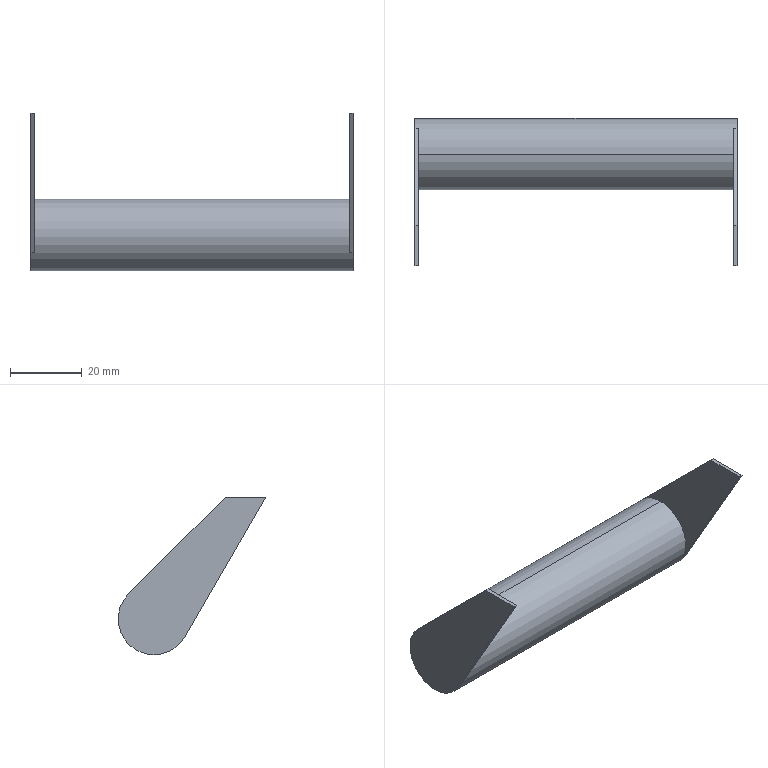Part | SolidWorks | features Extrusion 1, ICE 1, MirrorPattern 1 | 1 solid | 16 faces | box 90 x 41.177 x 44 mm | volume 6809 mm3 | plane 12 | cylinder 4 | commonest cylinder face diameters 18 x2 20 x2
STEP:
#1=CARTESIAN_POINT('',(45.,0.,-10.));
#2=VERTEX_POINT('',#1);
#3=CARTESIAN_POINT('',(45.,7.071,7.071));
#4=VERTEX_POINT('',#3);
#5=CARTESIAN_POINT('',(45.,0.,0.));
#6=DIRECTION('',(1.,0.,0.));
#7=DIRECTION('',(0.,0.,-1.));
#8=AXIS2_PLACEMENT_3D('',#5,#6,#7);
#9=CIRCLE('',#8,10.);
#10=EDGE_CURVE('',#2,#4,#9,.T.);
#11=ORIENTED_EDGE('',*,*,#10,.F.);
#12=CARTESIAN_POINT('',(-45.,0.,-10.));
#13=VERTEX_POINT('',#12);
#14=CARTESIAN_POINT('',(45.,0.,-10.));
#15=DIRECTION('',(-1.,0.,0.));
#16=VECTOR('',#15,1000.);
#17=LINE('',#14,#16);
#18=EDGE_CURVE('',#2,#13,#17,.T.);
#19=ORIENTED_EDGE('',*,*,#18,.T.);
#20=CARTESIAN_POINT('',(-45.,7.071,7.071));
#21=VERTEX_POINT('',#20);
#22=CARTESIAN_POINT('',(-45.,0.,0.));
#23=DIRECTION('',(1.,0.,0.));
#24=DIRECTION('',(0.,0.,-1.));
#25=AXIS2_PLACEMENT_3D('',#22,#23,#24);
#26=CIRCLE('',#25,10.);
#27=EDGE_CURVE('',#13,#21,#26,.T.);
#28=ORIENTED_EDGE('',*,*,#27,.T.);
#29=CARTESIAN_POINT('',(-44.,7.071,7.071));
#30=VERTEX_POINT('',#29);
#31=CARTESIAN_POINT('',(-44.,7.071,7.071));
#32=DIRECTION('',(-1.,0.,0.));
#33=VECTOR('',#32,1000.);
#34=LINE('',#31,#33);
#35=EDGE_CURVE('',#30,#21,#34,.T.);
#36=ORIENTED_EDGE('',*,*,#35,.F.);
#37=CARTESIAN_POINT('',(-44.,0.,10.));
#38=VERTEX_POINT('',#37);
#39=CARTESIAN_POINT('',(-44.,0.,0.));
#40=DIRECTION('',(-1.,0.,0.));
#41=DIRECTION('',(0.,0.,1.));
#42=AXIS2_PLACEMENT_3D('',#39,#40,#41);
#43=CIRCLE('',#42,10.);
#44=EDGE_CURVE('',#38,#30,#43,.T.);
#45=ORIENTED_EDGE('',*,*,#44,.F.);
#46=CARTESIAN_POINT('',(44.,0.,10.));
#47=VERTEX_POINT('',#46);
#48=CARTESIAN_POINT('',(45.,0.,10.));
#49=DIRECTION('',(-1.,0.,0.));
#50=VECTOR('',#49,1000.);
#51=LINE('',#48,#50);
#52=EDGE_CURVE('',#47,#38,#51,.T.);
#53=ORIENTED_EDGE('',*,*,#52,.F.);
#54=CARTESIAN_POINT('',(44.,7.071,7.071));
#55=VERTEX_POINT('',#54);
#56=CARTESIAN_POINT('',(44.,0.,0.));
#57=DIRECTION('',(1.,0.,0.));
#58=DIRECTION('',(0.,0.,-1.));
#59=AXIS2_PLACEMENT_3D('',#56,#57,#58);
#60=CIRCLE('',#59,10.);
#61=EDGE_CURVE('',#55,#47,#60,.T.);
#62=ORIENTED_EDGE('',*,*,#61,.F.);
#63=CARTESIAN_POINT('',(44.,7.071,7.071));
#64=DIRECTION('',(1.,0.,0.));
#65=VECTOR('',#64,1000.);
#66=LINE('',#63,#65);
#67=EDGE_CURVE('',#55,#4,#66,.T.);
#68=ORIENTED_EDGE('',*,*,#67,.T.);
#69=EDGE_LOOP('',(#11,#19,#28,#36,#45,#53,#62,#68));
#70=FACE_OUTER_BOUND('',#69,.T.);
#71=CARTESIAN_POINT('',(45.,0.,0.));
#72=DIRECTION('',(-1.,0.,0.));
#73=DIRECTION('',(0.,0.,1.));
#74=AXIS2_PLACEMENT_3D('',#71,#72,#73);
#75=CYLINDRICAL_SURFACE('',#74,10.);
#76=ADVANCED_FACE('',(#70),#75,.T.);
#77=ORIENTED_EDGE('',*,*,#18,.F.);
#78=CARTESIAN_POINT('',(45.,-8.66,-5.));
#79=VERTEX_POINT('',#78);
#80=CARTESIAN_POINT('',(45.,0.,0.));
#81=DIRECTION('',(1.,0.,0.));
#82=DIRECTION('',(0.,0.,-1.));
#83=AXIS2_PLACEMENT_3D('',#80,#81,#82);
#84=CIRCLE('',#83,10.);
#85=EDGE_CURVE('',#79,#2,#84,.T.);
#86=ORIENTED_EDGE('',*,*,#85,.F.);
#87=CARTESIAN_POINT('',(44.,-8.66,-5.));
#88=VERTEX_POINT('',#87);
#89=CARTESIAN_POINT('',(44.,-8.66,-5.));
#90=DIRECTION('',(1.,0.,0.));
#91=VECTOR('',#90,1000.);
#92=LINE('',#89,#91);
#93=EDGE_CURVE('',#88,#79,#92,.T.);
#94=ORIENTED_EDGE('',*,*,#93,.F.);
#95=CARTESIAN_POINT('',(44.,0.,0.));
#96=DIRECTION('',(1.,0.,0.));
#97=DIRECTION('',(0.,0.,-1.));
#98=AXIS2_PLACEMENT_3D('',#95,#96,#97);
#99=CIRCLE('',#98,10.);
#100=EDGE_CURVE('',#47,#88,#99,.T.);
#101=ORIENTED_EDGE('',*,*,#100,.F.);
#102=ORIENTED_EDGE('',*,*,#52,.T.);
#103=CARTESIAN_POINT('',(-44.,-8.66,-5.));
#104=VERTEX_POINT('',#103);
#105=CARTESIAN_POINT('',(-44.,0.,0.));
#106=DIRECTION('',(-1.,0.,0.));
#107=DIRECTION('',(0.,0.,1.));
#108=AXIS2_PLACEMENT_3D('',#105,#106,#107);
#109=CIRCLE('',#108,10.);
#110=EDGE_CURVE('',#104,#38,#109,.T.);
#111=ORIENTED_EDGE('',*,*,#110,.F.);
#112=CARTESIAN_POINT('',(-45.,-8.66,-5.));
#113=VERTEX_POINT('',#112);
#114=CARTESIAN_POINT('',(-44.,-8.66,-5.));
#115=DIRECTION('',(-1.,0.,0.));
#116=VECTOR('',#115,1000.);
#117=LINE('',#114,#116);
#118=EDGE_CURVE('',#104,#113,#117,.T.);
#119=ORIENTED_EDGE('',*,*,#118,.T.);
#120=CARTESIAN_POINT('',(-45.,0.,0.));
#121=DIRECTION('',(1.,0.,0.));
#122=DIRECTION('',(0.,0.,-1.));
#123=AXIS2_PLACEMENT_3D('',#120,#121,#122);
#124=CIRCLE('',#123,10.);
#125=EDGE_CURVE('',#113,#13,#124,.T.);
#126=ORIENTED_EDGE('',*,*,#125,.T.);
#127=EDGE_LOOP('',(#77,#86,#94,#101,#102,#111,#119,#126));
#128=FACE_OUTER_BOUND('',#127,.T.);
#129=CARTESIAN_POINT('',(45.,0.,0.));
#130=DIRECTION('',(-1.,0.,0.));
#131=DIRECTION('',(0.,0.,1.));
#132=AXIS2_PLACEMENT_3D('',#129,#130,#131);
#133=CYLINDRICAL_SURFACE('',#132,10.);
#134=ADVANCED_FACE('',(#128),#133,.T.);
#135=ORIENTED_EDGE('',*,*,#85,.T.);
#136=ORIENTED_EDGE('',*,*,#10,.T.);
#137=CARTESIAN_POINT('',(45.,-19.858,34.));
#138=VERTEX_POINT('',#137);
#139=CARTESIAN_POINT('',(45.,7.071,7.071));
#140=DIRECTION('',(0.,-0.7071,0.7071));
#141=VECTOR('',#140,1000.);
#142=LINE('',#139,#141);
#143=EDGE_CURVE('',#4,#138,#142,.T.);
#144=ORIENTED_EDGE('',*,*,#143,.T.);
#145=CARTESIAN_POINT('',(45.,-31.177,34.));
#146=VERTEX_POINT('',#145);
#147=CARTESIAN_POINT('',(45.,0.,34.));
#148=DIRECTION('',(0.,-1.,0.));
#149=VECTOR('',#148,1000.);
#150=LINE('',#147,#149);
#151=EDGE_CURVE('',#138,#146,#150,.T.);
#152=ORIENTED_EDGE('',*,*,#151,.T.);
#153=CARTESIAN_POINT('',(45.,-8.66,-5.));
#154=DIRECTION('',(0.,0.5,-0.866));
#155=VECTOR('',#154,1000.);
#156=LINE('',#153,#155);
#157=EDGE_CURVE('',#146,#79,#156,.T.);
#158=ORIENTED_EDGE('',*,*,#157,.T.);
#159=EDGE_LOOP('',(#135,#136,#144,#152,#158));
#160=FACE_OUTER_BOUND('',#159,.T.);
#161=CARTESIAN_POINT('',(45.,0.,0.));
#162=DIRECTION('',(1.,0.,0.));
#163=DIRECTION('',(0.,0.,-1.));
#164=AXIS2_PLACEMENT_3D('',#161,#162,#163);
#165=PLANE('',#164);
#166=ADVANCED_FACE('',(#160),#165,.T.);
#167=ORIENTED_EDGE('',*,*,#125,.F.);
#168=CARTESIAN_POINT('',(-45.,-31.177,34.));
#169=VERTEX_POINT('',#168);
#170=CARTESIAN_POINT('',(-45.,-8.66,-5.));
#171=DIRECTION('',(0.,0.5,-0.866));
#172=VECTOR('',#171,1000.);
#173=LINE('',#170,#172);
#174=EDGE_CURVE('',#169,#113,#173,.T.);
#175=ORIENTED_EDGE('',*,*,#174,.F.);
#176=CARTESIAN_POINT('',(-45.,-19.858,34.));
#177=VERTEX_POINT('',#176);
#178=CARTESIAN_POINT('',(-45.,0.,34.));
#179=DIRECTION('',(0.,-1.,0.));
#180=VECTOR('',#179,1000.);
#181=LINE('',#178,#180);
#182=EDGE_CURVE('',#177,#169,#181,.T.);
#183=ORIENTED_EDGE('',*,*,#182,.F.);
#184=CARTESIAN_POINT('',(-45.,7.071,7.071));
#185=DIRECTION('',(0.,-0.7071,0.7071));
#186=VECTOR('',#185,1000.);
#187=LINE('',#184,#186);
#188=EDGE_CURVE('',#21,#177,#187,.T.);
#189=ORIENTED_EDGE('',*,*,#188,.F.);
#190=ORIENTED_EDGE('',*,*,#27,.F.);
#191=EDGE_LOOP('',(#167,#175,#183,#189,#190));
#192=FACE_OUTER_BOUND('',#191,.T.);
#193=CARTESIAN_POINT('',(-45.,0.,0.));
#194=DIRECTION('',(1.,0.,0.));
#195=DIRECTION('',(0.,0.,-1.));
#196=AXIS2_PLACEMENT_3D('',#193,#194,#195);
#197=PLANE('',#196);
#198=ADVANCED_FACE('',(#192),#197,.F.);
#199=ORIENTED_EDGE('',*,*,#151,.F.);
#200=CARTESIAN_POINT('',(44.,-19.858,34.));
#201=VERTEX_POINT('',#200);
#202=CARTESIAN_POINT('',(44.,-19.858,34.));
#203=DIRECTION('',(1.,0.,0.));
#204=VECTOR('',#203,1000.);
#205=LINE('',#202,#204);
#206=EDGE_CURVE('',#201,#138,#205,.T.);
#207=ORIENTED_EDGE('',*,*,#206,.F.);
#208=CARTESIAN_POINT('',(44.,-31.177,34.));
#209=VERTEX_POINT('',#208);
#210=CARTESIAN_POINT('',(44.,0.,34.));
#211=DIRECTION('',(0.,-1.,0.));
#212=VECTOR('',#211,1000.);
#213=LINE('',#210,#212);
#214=EDGE_CURVE('',#201,#209,#213,.T.);
#215=ORIENTED_EDGE('',*,*,#214,.T.);
#216=CARTESIAN_POINT('',(44.,-31.177,34.));
#217=DIRECTION('',(1.,0.,0.));
#218=VECTOR('',#217,1000.);
#219=LINE('',#216,#218);
#220=EDGE_CURVE('',#209,#146,#219,.T.);
#221=ORIENTED_EDGE('',*,*,#220,.T.);
#222=EDGE_LOOP('',(#199,#207,#215,#221));
#223=FACE_OUTER_BOUND('',#222,.T.);
#224=CARTESIAN_POINT('',(44.,0.,34.));
#225=DIRECTION('',(0.,0.,1.));
#226=DIRECTION('',(1.,0.,0.));
#227=AXIS2_PLACEMENT_3D('',#224,#225,#226);
#228=PLANE('',#227);
#229=ADVANCED_FACE('',(#223),#228,.T.);
#230=ORIENTED_EDGE('',*,*,#143,.F.);
#231=ORIENTED_EDGE('',*,*,#67,.F.);
#232=CARTESIAN_POINT('',(44.,7.071,7.071));
#233=DIRECTION('',(0.,-0.7071,0.7071));
#234=VECTOR('',#233,1000.);
#235=LINE('',#232,#234);
#236=EDGE_CURVE('',#55,#201,#235,.T.);
#237=ORIENTED_EDGE('',*,*,#236,.T.);
#238=ORIENTED_EDGE('',*,*,#206,.T.);
#239=EDGE_LOOP('',(#230,#231,#237,#238));
#240=FACE_OUTER_BOUND('',#239,.T.);
#241=CARTESIAN_POINT('',(44.,7.071,7.071));
#242=DIRECTION('',(0.,0.7071,0.7071));
#243=DIRECTION('',(0.,-0.7071,0.7071));
#244=AXIS2_PLACEMENT_3D('',#241,#242,#243);
#245=PLANE('',#244);
#246=ADVANCED_FACE('',(#240),#245,.T.);
#247=ORIENTED_EDGE('',*,*,#157,.F.);
#248=ORIENTED_EDGE('',*,*,#220,.F.);
#249=CARTESIAN_POINT('',(44.,-8.66,-5.));
#250=DIRECTION('',(0.,0.5,-0.866));
#251=VECTOR('',#250,1000.);
#252=LINE('',#249,#251);
#253=EDGE_CURVE('',#209,#88,#252,.T.);
#254=ORIENTED_EDGE('',*,*,#253,.T.);
#255=ORIENTED_EDGE('',*,*,#93,.T.);
#256=EDGE_LOOP('',(#247,#248,#254,#255));
#257=FACE_OUTER_BOUND('',#256,.T.);
#258=CARTESIAN_POINT('',(44.,-8.66,-5.));
#259=DIRECTION('',(0.,-0.866,-0.5));
#260=DIRECTION('',(0.,0.5,-0.866));
#261=AXIS2_PLACEMENT_3D('',#258,#259,#260);
#262=PLANE('',#261);
#263=ADVANCED_FACE('',(#257),#262,.T.);
#264=ORIENTED_EDGE('',*,*,#236,.F.);
#265=ORIENTED_EDGE('',*,*,#61,.T.);
#266=ORIENTED_EDGE('',*,*,#100,.T.);
#267=ORIENTED_EDGE('',*,*,#253,.F.);
#268=ORIENTED_EDGE('',*,*,#214,.F.);
#269=EDGE_LOOP('',(#264,#265,#266,#267,#268));
#270=FACE_OUTER_BOUND('',#269,.T.);
#271=CARTESIAN_POINT('',(44.,0.,0.));
#272=DIRECTION('',(1.,0.,0.));
#273=DIRECTION('',(0.,0.,-1.));
#274=AXIS2_PLACEMENT_3D('',#271,#272,#273);
#275=PLANE('',#274);
#276=ADVANCED_FACE('',(#270),#275,.F.);
#277=ORIENTED_EDGE('',*,*,#182,.T.);
#278=CARTESIAN_POINT('',(-44.,-31.177,34.));
#279=VERTEX_POINT('',#278);
#280=CARTESIAN_POINT('',(-44.,-31.177,34.));
#281=DIRECTION('',(-1.,0.,0.));
#282=VECTOR('',#281,1000.);
#283=LINE('',#280,#282);
#284=EDGE_CURVE('',#279,#169,#283,.T.);
#285=ORIENTED_EDGE('',*,*,#284,.F.);
#286=CARTESIAN_POINT('',(-44.,-19.858,34.));
#287=VERTEX_POINT('',#286);
#288=CARTESIAN_POINT('',(-44.,0.,34.));
#289=DIRECTION('',(0.,-1.,0.));
#290=VECTOR('',#289,1000.);
#291=LINE('',#288,#290);
#292=EDGE_CURVE('',#287,#279,#291,.T.);
#293=ORIENTED_EDGE('',*,*,#292,.F.);
#294=CARTESIAN_POINT('',(-44.,-19.858,34.));
#295=DIRECTION('',(-1.,0.,0.));
#296=VECTOR('',#295,1000.);
#297=LINE('',#294,#296);
#298=EDGE_CURVE('',#287,#177,#297,.T.);
#299=ORIENTED_EDGE('',*,*,#298,.T.);
#300=EDGE_LOOP('',(#277,#285,#293,#299));
#301=FACE_OUTER_BOUND('',#300,.T.);
#302=CARTESIAN_POINT('',(-44.,0.,34.));
#303=DIRECTION('',(0.,0.,-1.));
#304=DIRECTION('',(-1.,0.,0.));
#305=AXIS2_PLACEMENT_3D('',#302,#303,#304);
#306=PLANE('',#305);
#307=ADVANCED_FACE('',(#301),#306,.F.);
#308=ORIENTED_EDGE('',*,*,#174,.T.);
#309=ORIENTED_EDGE('',*,*,#118,.F.);
#310=CARTESIAN_POINT('',(-44.,-8.66,-5.));
#311=DIRECTION('',(0.,0.5,-0.866));
#312=VECTOR('',#311,1000.);
#313=LINE('',#310,#312);
#314=EDGE_CURVE('',#279,#104,#313,.T.);
#315=ORIENTED_EDGE('',*,*,#314,.F.);
#316=ORIENTED_EDGE('',*,*,#284,.T.);
#317=EDGE_LOOP('',(#308,#309,#315,#316));
#318=FACE_OUTER_BOUND('',#317,.T.);
#319=CARTESIAN_POINT('',(-44.,-8.66,-5.));
#320=DIRECTION('',(0.,0.866,0.5));
#321=DIRECTION('',(0.,-0.5,0.866));
#322=AXIS2_PLACEMENT_3D('',#319,#320,#321);
#323=PLANE('',#322);
#324=ADVANCED_FACE('',(#318),#323,.F.);
#325=ORIENTED_EDGE('',*,*,#188,.T.);
#326=ORIENTED_EDGE('',*,*,#298,.F.);
#327=CARTESIAN_POINT('',(-44.,7.071,7.071));
#328=DIRECTION('',(0.,-0.7071,0.7071));
#329=VECTOR('',#328,1000.);
#330=LINE('',#327,#329);
#331=EDGE_CURVE('',#30,#287,#330,.T.);
#332=ORIENTED_EDGE('',*,*,#331,.F.);
#333=ORIENTED_EDGE('',*,*,#35,.T.);
#334=EDGE_LOOP('',(#325,#326,#332,#333));
#335=FACE_OUTER_BOUND('',#334,.T.);
#336=CARTESIAN_POINT('',(-44.,7.071,7.071));
#337=DIRECTION('',(0.,-0.7071,-0.7071));
#338=DIRECTION('',(0.,0.7071,-0.7071));
#339=AXIS2_PLACEMENT_3D('',#336,#337,#338);
#340=PLANE('',#339);
#341=ADVANCED_FACE('',(#335),#340,.F.);
#342=ORIENTED_EDGE('',*,*,#314,.T.);
#343=ORIENTED_EDGE('',*,*,#110,.T.);
#344=ORIENTED_EDGE('',*,*,#44,.T.);
#345=ORIENTED_EDGE('',*,*,#331,.T.);
#346=ORIENTED_EDGE('',*,*,#292,.T.);
#347=EDGE_LOOP('',(#342,#343,#344,#345,#346));
#348=FACE_OUTER_BOUND('',#347,.T.);
#349=CARTESIAN_POINT('',(-44.,0.,0.));
#350=DIRECTION('',(-1.,0.,0.));
#351=DIRECTION('',(0.,0.,-1.));
#352=AXIS2_PLACEMENT_3D('',#349,#350,#351);
#353=PLANE('',#352);
#354=ADVANCED_FACE('',(#348),#353,.F.);
#355=CLOSED_SHELL('',(#76,#134,#166,#198,#229,#246,#263,#276,#307,#324,#341,#354));
#356=CARTESIAN_POINT('',(44.,0.,9.));
#357=VERTEX_POINT('',#356);
#358=CARTESIAN_POINT('',(44.,0.,-9.));
#359=VERTEX_POINT('',#358);
#360=CARTESIAN_POINT('',(44.,0.,0.));
#361=DIRECTION('',(1.,0.,0.));
#362=DIRECTION('',(0.,0.,-1.));
#363=AXIS2_PLACEMENT_3D('',#360,#361,#362);
#364=CIRCLE('',#363,9.);
#365=EDGE_CURVE('',#357,#359,#364,.T.);
#366=ORIENTED_EDGE('',*,*,#365,.T.);
#367=CARTESIAN_POINT('',(-44.,0.,-9.));
#368=VERTEX_POINT('',#367);
#369=CARTESIAN_POINT('',(45.,0.,-9.));
#370=DIRECTION('',(-1.,0.,0.));
#371=VECTOR('',#370,1000.);
#372=LINE('',#369,#371);
#373=EDGE_CURVE('',#359,#368,#372,.T.);
#374=ORIENTED_EDGE('',*,*,#373,.T.);
#375=CARTESIAN_POINT('',(-44.,0.,9.));
#376=VERTEX_POINT('',#375);
#377=CARTESIAN_POINT('',(-44.,0.,0.));
#378=DIRECTION('',(-1.,0.,0.));
#379=DIRECTION('',(0.,0.,1.));
#380=AXIS2_PLACEMENT_3D('',#377,#378,#379);
#381=CIRCLE('',#380,9.);
#382=EDGE_CURVE('',#368,#376,#381,.T.);
#383=ORIENTED_EDGE('',*,*,#382,.T.);
#384=CARTESIAN_POINT('',(45.,0.,9.));
#385=DIRECTION('',(-1.,0.,0.));
#386=VECTOR('',#385,1000.);
#387=LINE('',#384,#386);
#388=EDGE_CURVE('',#357,#376,#387,.T.);
#389=ORIENTED_EDGE('',*,*,#388,.F.);
#390=EDGE_LOOP('',(#366,#374,#383,#389));
#391=FACE_OUTER_BOUND('',#390,.T.);
#392=CARTESIAN_POINT('',(45.,0.,0.));
#393=DIRECTION('',(-1.,0.,0.));
#394=DIRECTION('',(0.,0.,1.));
#395=AXIS2_PLACEMENT_3D('',#392,#393,#394);
#396=CYLINDRICAL_SURFACE('',#395,9.);
#397=ADVANCED_FACE('',(#391),#396,.F.);
#398=ORIENTED_EDGE('',*,*,#365,.F.);
#399=CARTESIAN_POINT('',(44.,0.,0.));
#400=DIRECTION('',(1.,0.,0.));
#401=DIRECTION('',(0.,0.,-1.));
#402=AXIS2_PLACEMENT_3D('',#399,#400,#401);
#403=CIRCLE('',#402,9.);
#404=EDGE_CURVE('',#359,#357,#403,.T.);
#405=ORIENTED_EDGE('',*,*,#404,.F.);
#406=EDGE_LOOP('',(#398,#405));
#407=FACE_OUTER_BOUND('',#406,.T.);
#408=CARTESIAN_POINT('',(44.,0.,0.));
#409=DIRECTION('',(1.,0.,0.));
#410=DIRECTION('',(0.,0.,-1.));
#411=AXIS2_PLACEMENT_3D('',#408,#409,#410);
#412=PLANE('',#411);
#413=ADVANCED_FACE('',(#407),#412,.F.);
#414=ORIENTED_EDGE('',*,*,#373,.F.);
#415=ORIENTED_EDGE('',*,*,#404,.T.);
#416=ORIENTED_EDGE('',*,*,#388,.T.);
#417=CARTESIAN_POINT('',(-44.,0.,0.));
#418=DIRECTION('',(-1.,0.,0.));
#419=DIRECTION('',(0.,0.,1.));
#420=AXIS2_PLACEMENT_3D('',#417,#418,#419);
#421=CIRCLE('',#420,9.);
#422=EDGE_CURVE('',#376,#368,#421,.T.);
#423=ORIENTED_EDGE('',*,*,#422,.T.);
#424=EDGE_LOOP('',(#414,#415,#416,#423));
#425=FACE_OUTER_BOUND('',#424,.T.);
#426=CARTESIAN_POINT('',(45.,0.,0.));
#427=DIRECTION('',(-1.,0.,0.));
#428=DIRECTION('',(0.,0.,1.));
#429=AXIS2_PLACEMENT_3D('',#426,#427,#428);
#430=CYLINDRICAL_SURFACE('',#429,9.);
#431=ADVANCED_FACE('',(#425),#430,.F.);
#432=ORIENTED_EDGE('',*,*,#422,.F.);
#433=ORIENTED_EDGE('',*,*,#382,.F.);
#434=EDGE_LOOP('',(#432,#433));
#435=FACE_OUTER_BOUND('',#434,.T.);
#436=CARTESIAN_POINT('',(-44.,0.,0.));
#437=DIRECTION('',(-1.,0.,0.));
#438=DIRECTION('',(0.,0.,-1.));
#439=AXIS2_PLACEMENT_3D('',#436,#437,#438);
#440=PLANE('',#439);
#441=ADVANCED_FACE('',(#435),#440,.F.);
#442=CLOSED_SHELL('',(#397,#413,#431,#441));
#443=ORIENTED_CLOSED_SHELL('',*,#442,.F.);
#444=BREP_WITH_VOIDS('',#355,(#443));
#445=CARTESIAN_POINT('',(0.,0.,0.));
#446=DIRECTION('',(0.,0.,1.));
#447=DIRECTION('',(1.,0.,0.));
#448=AXIS2_PLACEMENT_3D('',#445,#446,#447);
#449=(LENGTH_UNIT()NAMED_UNIT(*)SI_UNIT(.MILLI.,.METRE.));
#450=UNCERTAINTY_MEASURE_WITH_UNIT(LENGTH_MEASURE(0.00001),#449,'','');
#451=(NAMED_UNIT(*)PLANE_ANGLE_UNIT()SI_UNIT($,.RADIAN.));
#452=(NAMED_UNIT(*)SI_UNIT($,.STERADIAN.)SOLID_ANGLE_UNIT());
#453=(GEOMETRIC_REPRESENTATION_CONTEXT(3)GLOBAL_UNCERTAINTY_ASSIGNED_CONTEXT((#450))GLOBAL_UNIT_ASSIGNED_CONTEXT((#449,#451,#452))REPRESENTATION_CONTEXT('',''));
#454=ADVANCED_BREP_SHAPE_REPRESENTATION('',(#444,#448),#453);